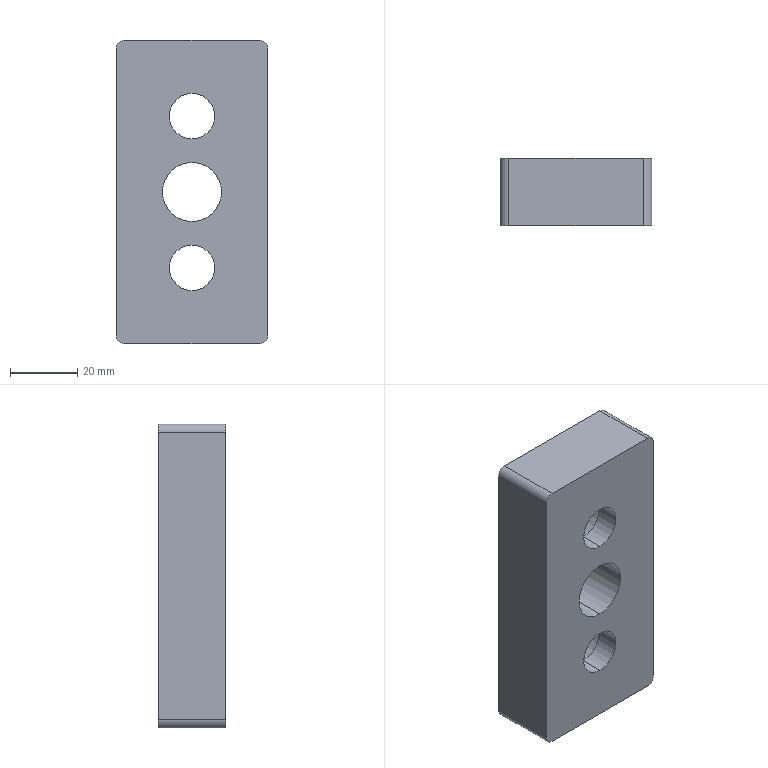Part | STEP file | PN_0027 | 1 solid | 22 faces | box 45 x 20 x 90 mm | volume 65910 mm3 | cylinder 14 | plane 8 | commonest cylinder face diameters 5 x4 13.5 x4 20 x4 17.5 x2